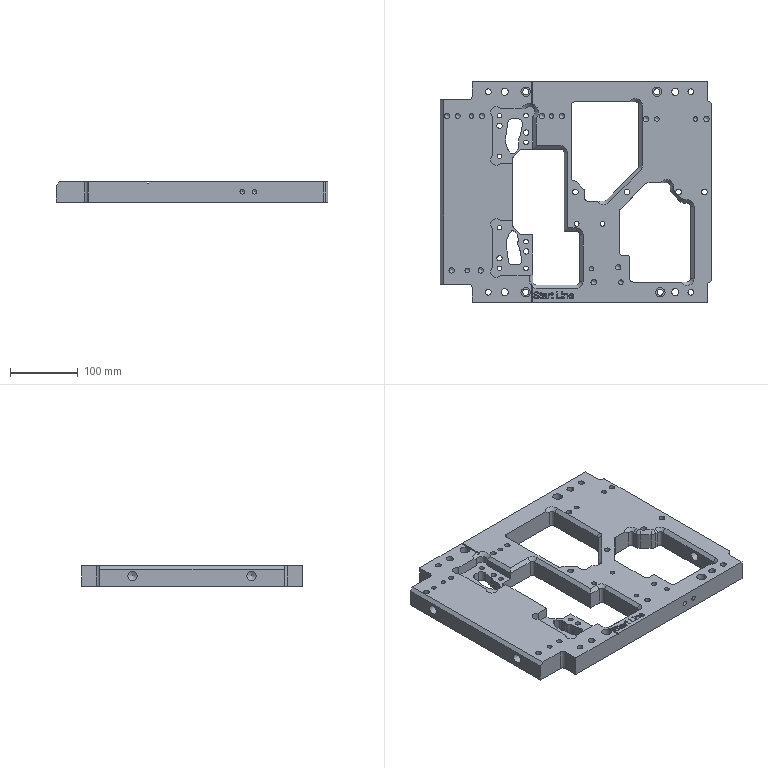Part | STEP file | 1 solid | 434 faces | box 400 x 325 x 30 mm | volume 2323925 mm3 | plane 154 | cylinder 124 | other 116 | cone 36 | spline 4 | commonest cylinder face diameters 10 x29 6.8 x18 8 x15 14 x10 8.5 x8 20 x6